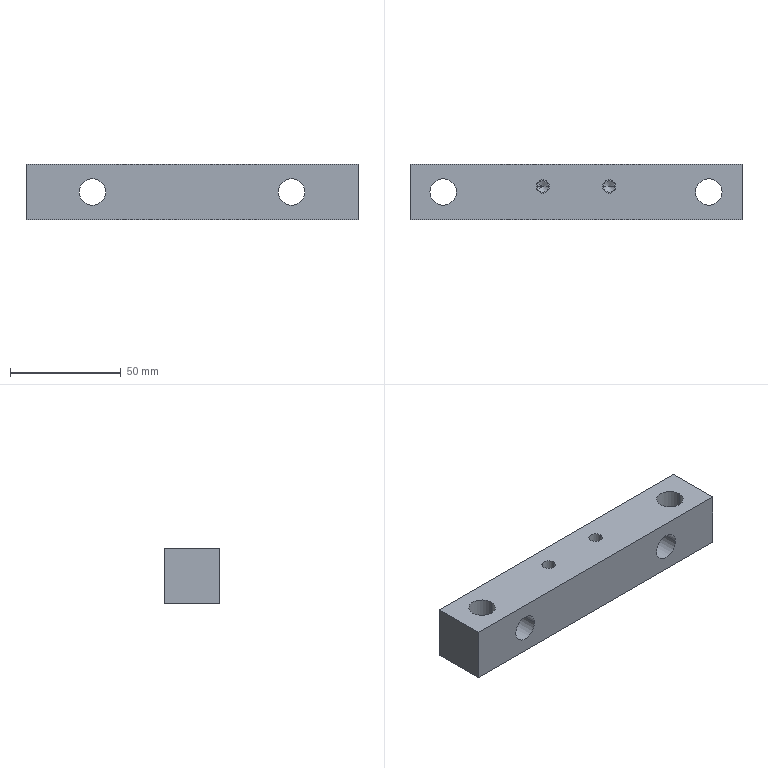Part | STEP file | J013-EBZ05-28-06-Part-1 | 1 solid | 28 faces | box 150 x 25 x 25 mm | volume 81414 mm3 | cylinder 16 | plane 8 | cone 4 | commonest cylinder face diameters 12 x8 5.1 x4 6 x4
STEP:
#1=CARTESIAN_POINT('',(90.,15.,3.468));
#2=VERTEX_POINT('',#1);
#3=CARTESIAN_POINT('',(87.45,15.,5.));
#4=VERTEX_POINT('',#3);
#5=CARTESIAN_POINT('',(87.45,15.,5.));
#6=DIRECTION('',(-0.8572,0.,0.515));
#7=VECTOR('',#6,1000.);
#8=LINE('',#5,#7);
#9=EDGE_CURVE('',#2,#4,#8,.T.);
#10=ORIENTED_EDGE('',*,*,#9,.F.);
#11=CARTESIAN_POINT('',(92.55,15.,5.));
#12=VERTEX_POINT('',#11);
#13=CARTESIAN_POINT('',(92.55,15.,5.));
#14=DIRECTION('',(0.8572,0.,0.515));
#15=VECTOR('',#14,1000.);
#16=LINE('',#13,#15);
#17=EDGE_CURVE('',#2,#12,#16,.T.);
#18=ORIENTED_EDGE('',*,*,#17,.T.);
#19=CARTESIAN_POINT('',(90.,15.,5.));
#20=DIRECTION('',(0.,0.,1.));
#21=DIRECTION('',(-1.,0.,0.));
#22=AXIS2_PLACEMENT_3D('',#19,#20,#21);
#23=CIRCLE('',#22,2.55);
#24=EDGE_CURVE('',#12,#4,#23,.T.);
#25=ORIENTED_EDGE('',*,*,#24,.T.);
#26=EDGE_LOOP('',(#10,#18,#25));
#27=FACE_OUTER_BOUND('',#26,.T.);
#28=CARTESIAN_POINT('',(90.,15.,5.));
#29=DIRECTION('',(0.,0.,1.));
#30=DIRECTION('',(-1.,0.,0.));
#31=AXIS2_PLACEMENT_3D('',#28,#29,#30);
#32=CONICAL_SURFACE('',#31,2.55,1.03);
#33=ADVANCED_FACE('',(#27),#32,.F.);
#34=ORIENTED_EDGE('',*,*,#24,.F.);
#35=CARTESIAN_POINT('',(92.55,15.,13.));
#36=VERTEX_POINT('',#35);
#37=CARTESIAN_POINT('',(92.55,15.,25.));
#38=DIRECTION('',(0.,0.,1.));
#39=VECTOR('',#38,1000.);
#40=LINE('',#37,#39);
#41=EDGE_CURVE('',#12,#36,#40,.T.);
#42=ORIENTED_EDGE('',*,*,#41,.T.);
#43=CARTESIAN_POINT('',(87.45,15.,13.));
#44=VERTEX_POINT('',#43);
#45=CARTESIAN_POINT('',(90.,15.,13.));
#46=DIRECTION('',(0.,0.,1.));
#47=DIRECTION('',(-1.,0.,0.));
#48=AXIS2_PLACEMENT_3D('',#45,#46,#47);
#49=CIRCLE('',#48,2.55);
#50=EDGE_CURVE('',#36,#44,#49,.T.);
#51=ORIENTED_EDGE('',*,*,#50,.T.);
#52=CARTESIAN_POINT('',(87.45,15.,25.));
#53=DIRECTION('',(0.,0.,1.));
#54=VECTOR('',#53,1000.);
#55=LINE('',#52,#54);
#56=EDGE_CURVE('',#4,#44,#55,.T.);
#57=ORIENTED_EDGE('',*,*,#56,.F.);
#58=EDGE_LOOP('',(#34,#42,#51,#57));
#59=FACE_OUTER_BOUND('',#58,.T.);
#60=CARTESIAN_POINT('',(90.,15.,25.));
#61=DIRECTION('',(0.,0.,1.));
#62=DIRECTION('',(-1.,0.,0.));
#63=AXIS2_PLACEMENT_3D('',#60,#61,#62);
#64=CYLINDRICAL_SURFACE('',#63,2.55);
#65=ADVANCED_FACE('',(#59),#64,.F.);
#66=CARTESIAN_POINT('',(93.,15.,13.));
#67=VERTEX_POINT('',#66);
#68=CARTESIAN_POINT('',(87.,15.,13.));
#69=VERTEX_POINT('',#68);
#70=CARTESIAN_POINT('',(90.,15.,13.));
#71=DIRECTION('',(0.,0.,1.));
#72=DIRECTION('',(-1.,0.,0.));
#73=AXIS2_PLACEMENT_3D('',#70,#71,#72);
#74=CIRCLE('',#73,3.);
#75=EDGE_CURVE('',#67,#69,#74,.T.);
#76=ORIENTED_EDGE('',*,*,#75,.F.);
#77=CARTESIAN_POINT('',(93.,15.,25.));
#78=VERTEX_POINT('',#77);
#79=CARTESIAN_POINT('',(93.,15.,25.));
#80=DIRECTION('',(0.,0.,1.));
#81=VECTOR('',#80,1000.);
#82=LINE('',#79,#81);
#83=EDGE_CURVE('',#67,#78,#82,.T.);
#84=ORIENTED_EDGE('',*,*,#83,.T.);
#85=CARTESIAN_POINT('',(87.,15.,25.));
#86=VERTEX_POINT('',#85);
#87=CARTESIAN_POINT('',(90.,15.,25.));
#88=DIRECTION('',(0.,0.,1.));
#89=DIRECTION('',(-1.,0.,0.));
#90=AXIS2_PLACEMENT_3D('',#87,#88,#89);
#91=CIRCLE('',#90,3.);
#92=EDGE_CURVE('',#78,#86,#91,.T.);
#93=ORIENTED_EDGE('',*,*,#92,.T.);
#94=CARTESIAN_POINT('',(87.,15.,25.));
#95=DIRECTION('',(0.,0.,1.));
#96=VECTOR('',#95,1000.);
#97=LINE('',#94,#96);
#98=EDGE_CURVE('',#69,#86,#97,.T.);
#99=ORIENTED_EDGE('',*,*,#98,.F.);
#100=EDGE_LOOP('',(#76,#84,#93,#99));
#101=FACE_OUTER_BOUND('',#100,.T.);
#102=CARTESIAN_POINT('',(90.,15.,25.));
#103=DIRECTION('',(0.,0.,1.));
#104=DIRECTION('',(-1.,0.,0.));
#105=AXIS2_PLACEMENT_3D('',#102,#103,#104);
#106=CYLINDRICAL_SURFACE('',#105,3.);
#107=ADVANCED_FACE('',(#101),#106,.F.);
#108=CARTESIAN_POINT('',(60.,15.,3.468));
#109=VERTEX_POINT('',#108);
#110=CARTESIAN_POINT('',(57.45,15.,5.));
#111=VERTEX_POINT('',#110);
#112=CARTESIAN_POINT('',(57.45,15.,5.));
#113=DIRECTION('',(-0.8572,0.,0.515));
#114=VECTOR('',#113,1000.);
#115=LINE('',#112,#114);
#116=EDGE_CURVE('',#109,#111,#115,.T.);
#117=ORIENTED_EDGE('',*,*,#116,.F.);
#118=CARTESIAN_POINT('',(62.55,15.,5.));
#119=VERTEX_POINT('',#118);
#120=CARTESIAN_POINT('',(62.55,15.,5.));
#121=DIRECTION('',(0.8572,0.,0.515));
#122=VECTOR('',#121,1000.);
#123=LINE('',#120,#122);
#124=EDGE_CURVE('',#109,#119,#123,.T.);
#125=ORIENTED_EDGE('',*,*,#124,.T.);
#126=CARTESIAN_POINT('',(60.,15.,5.));
#127=DIRECTION('',(0.,0.,1.));
#128=DIRECTION('',(-1.,0.,0.));
#129=AXIS2_PLACEMENT_3D('',#126,#127,#128);
#130=CIRCLE('',#129,2.55);
#131=EDGE_CURVE('',#119,#111,#130,.T.);
#132=ORIENTED_EDGE('',*,*,#131,.T.);
#133=EDGE_LOOP('',(#117,#125,#132));
#134=FACE_OUTER_BOUND('',#133,.T.);
#135=CARTESIAN_POINT('',(60.,15.,5.));
#136=DIRECTION('',(0.,0.,1.));
#137=DIRECTION('',(-1.,0.,0.));
#138=AXIS2_PLACEMENT_3D('',#135,#136,#137);
#139=CONICAL_SURFACE('',#138,2.55,1.03);
#140=ADVANCED_FACE('',(#134),#139,.F.);
#141=ORIENTED_EDGE('',*,*,#131,.F.);
#142=CARTESIAN_POINT('',(62.55,15.,13.));
#143=VERTEX_POINT('',#142);
#144=CARTESIAN_POINT('',(62.55,15.,25.));
#145=DIRECTION('',(0.,0.,1.));
#146=VECTOR('',#145,1000.);
#147=LINE('',#144,#146);
#148=EDGE_CURVE('',#119,#143,#147,.T.);
#149=ORIENTED_EDGE('',*,*,#148,.T.);
#150=CARTESIAN_POINT('',(57.45,15.,13.));
#151=VERTEX_POINT('',#150);
#152=CARTESIAN_POINT('',(60.,15.,13.));
#153=DIRECTION('',(0.,0.,1.));
#154=DIRECTION('',(-1.,0.,0.));
#155=AXIS2_PLACEMENT_3D('',#152,#153,#154);
#156=CIRCLE('',#155,2.55);
#157=EDGE_CURVE('',#143,#151,#156,.T.);
#158=ORIENTED_EDGE('',*,*,#157,.T.);
#159=CARTESIAN_POINT('',(57.45,15.,25.));
#160=DIRECTION('',(0.,0.,1.));
#161=VECTOR('',#160,1000.);
#162=LINE('',#159,#161);
#163=EDGE_CURVE('',#111,#151,#162,.T.);
#164=ORIENTED_EDGE('',*,*,#163,.F.);
#165=EDGE_LOOP('',(#141,#149,#158,#164));
#166=FACE_OUTER_BOUND('',#165,.T.);
#167=CARTESIAN_POINT('',(60.,15.,25.));
#168=DIRECTION('',(0.,0.,1.));
#169=DIRECTION('',(-1.,0.,0.));
#170=AXIS2_PLACEMENT_3D('',#167,#168,#169);
#171=CYLINDRICAL_SURFACE('',#170,2.55);
#172=ADVANCED_FACE('',(#166),#171,.F.);
#173=CARTESIAN_POINT('',(63.,15.,13.));
#174=VERTEX_POINT('',#173);
#175=CARTESIAN_POINT('',(57.,15.,13.));
#176=VERTEX_POINT('',#175);
#177=CARTESIAN_POINT('',(60.,15.,13.));
#178=DIRECTION('',(0.,0.,1.));
#179=DIRECTION('',(-1.,0.,0.));
#180=AXIS2_PLACEMENT_3D('',#177,#178,#179);
#181=CIRCLE('',#180,3.);
#182=EDGE_CURVE('',#174,#176,#181,.T.);
#183=ORIENTED_EDGE('',*,*,#182,.F.);
#184=CARTESIAN_POINT('',(63.,15.,25.));
#185=VERTEX_POINT('',#184);
#186=CARTESIAN_POINT('',(63.,15.,25.));
#187=DIRECTION('',(0.,0.,1.));
#188=VECTOR('',#187,1000.);
#189=LINE('',#186,#188);
#190=EDGE_CURVE('',#174,#185,#189,.T.);
#191=ORIENTED_EDGE('',*,*,#190,.T.);
#192=CARTESIAN_POINT('',(57.,15.,25.));
#193=VERTEX_POINT('',#192);
#194=CARTESIAN_POINT('',(60.,15.,25.));
#195=DIRECTION('',(0.,0.,1.));
#196=DIRECTION('',(-1.,0.,0.));
#197=AXIS2_PLACEMENT_3D('',#194,#195,#196);
#198=CIRCLE('',#197,3.);
#199=EDGE_CURVE('',#185,#193,#198,.T.);
#200=ORIENTED_EDGE('',*,*,#199,.T.);
#201=CARTESIAN_POINT('',(57.,15.,25.));
#202=DIRECTION('',(0.,0.,1.));
#203=VECTOR('',#202,1000.);
#204=LINE('',#201,#203);
#205=EDGE_CURVE('',#176,#193,#204,.T.);
#206=ORIENTED_EDGE('',*,*,#205,.F.);
#207=EDGE_LOOP('',(#183,#191,#200,#206));
#208=FACE_OUTER_BOUND('',#207,.T.);
#209=CARTESIAN_POINT('',(60.,15.,25.));
#210=DIRECTION('',(0.,0.,1.));
#211=DIRECTION('',(-1.,0.,0.));
#212=AXIS2_PLACEMENT_3D('',#209,#210,#211);
#213=CYLINDRICAL_SURFACE('',#212,3.);
#214=ADVANCED_FACE('',(#208),#213,.F.);
#215=CARTESIAN_POINT('',(114.,25.,12.5));
#216=VERTEX_POINT('',#215);
#217=CARTESIAN_POINT('',(126.,25.,12.5));
#218=VERTEX_POINT('',#217);
#219=CARTESIAN_POINT('',(120.,25.,12.5));
#220=DIRECTION('',(0.,-1.,0.));
#221=DIRECTION('',(1.,0.,0.));
#222=AXIS2_PLACEMENT_3D('',#219,#220,#221);
#223=CIRCLE('',#222,6.);
#224=EDGE_CURVE('',#216,#218,#223,.T.);
#225=ORIENTED_EDGE('',*,*,#224,.F.);
#226=CARTESIAN_POINT('',(114.,0.,12.5));
#227=VERTEX_POINT('',#226);
#228=CARTESIAN_POINT('',(114.,25.,12.5));
#229=DIRECTION('',(0.,-1.,0.));
#230=VECTOR('',#229,1000.);
#231=LINE('',#228,#230);
#232=EDGE_CURVE('',#216,#227,#231,.T.);
#233=ORIENTED_EDGE('',*,*,#232,.T.);
#234=CARTESIAN_POINT('',(126.,0.,12.5));
#235=VERTEX_POINT('',#234);
#236=CARTESIAN_POINT('',(120.,0.,12.5));
#237=DIRECTION('',(0.,1.,0.));
#238=DIRECTION('',(-1.,0.,0.));
#239=AXIS2_PLACEMENT_3D('',#236,#237,#238);
#240=CIRCLE('',#239,6.);
#241=EDGE_CURVE('',#235,#227,#240,.T.);
#242=ORIENTED_EDGE('',*,*,#241,.F.);
#243=CARTESIAN_POINT('',(126.,25.,12.5));
#244=DIRECTION('',(0.,-1.,0.));
#245=VECTOR('',#244,1000.);
#246=LINE('',#243,#245);
#247=EDGE_CURVE('',#218,#235,#246,.T.);
#248=ORIENTED_EDGE('',*,*,#247,.F.);
#249=EDGE_LOOP('',(#225,#233,#242,#248));
#250=FACE_OUTER_BOUND('',#249,.T.);
#251=CARTESIAN_POINT('',(120.,25.,12.5));
#252=DIRECTION('',(0.,-1.,0.));
#253=DIRECTION('',(1.,0.,0.));
#254=AXIS2_PLACEMENT_3D('',#251,#252,#253);
#255=CYLINDRICAL_SURFACE('',#254,6.);
#256=ADVANCED_FACE('',(#250),#255,.F.);
#257=CARTESIAN_POINT('',(129.,12.5,25.));
#258=VERTEX_POINT('',#257);
#259=CARTESIAN_POINT('',(141.,12.5,25.));
#260=VERTEX_POINT('',#259);
#261=CARTESIAN_POINT('',(135.,12.5,25.));
#262=DIRECTION('',(0.,0.,-1.));
#263=DIRECTION('',(1.,0.,0.));
#264=AXIS2_PLACEMENT_3D('',#261,#262,#263);
#265=CIRCLE('',#264,6.);
#266=EDGE_CURVE('',#258,#260,#265,.T.);
#267=ORIENTED_EDGE('',*,*,#266,.F.);
#268=CARTESIAN_POINT('',(129.,12.5,0.));
#269=VERTEX_POINT('',#268);
#270=CARTESIAN_POINT('',(129.,12.5,25.));
#271=DIRECTION('',(0.,0.,-1.));
#272=VECTOR('',#271,1000.);
#273=LINE('',#270,#272);
#274=EDGE_CURVE('',#258,#269,#273,.T.);
#275=ORIENTED_EDGE('',*,*,#274,.T.);
#276=CARTESIAN_POINT('',(141.,12.5,0.));
#277=VERTEX_POINT('',#276);
#278=CARTESIAN_POINT('',(135.,12.5,0.));
#279=DIRECTION('',(0.,0.,1.));
#280=DIRECTION('',(-1.,0.,0.));
#281=AXIS2_PLACEMENT_3D('',#278,#279,#280);
#282=CIRCLE('',#281,6.);
#283=EDGE_CURVE('',#277,#269,#282,.T.);
#284=ORIENTED_EDGE('',*,*,#283,.F.);
#285=CARTESIAN_POINT('',(141.,12.5,25.));
#286=DIRECTION('',(0.,0.,-1.));
#287=VECTOR('',#286,1000.);
#288=LINE('',#285,#287);
#289=EDGE_CURVE('',#260,#277,#288,.T.);
#290=ORIENTED_EDGE('',*,*,#289,.F.);
#291=EDGE_LOOP('',(#267,#275,#284,#290));
#292=FACE_OUTER_BOUND('',#291,.T.);
#293=CARTESIAN_POINT('',(135.,12.5,25.));
#294=DIRECTION('',(0.,0.,-1.));
#295=DIRECTION('',(1.,0.,0.));
#296=AXIS2_PLACEMENT_3D('',#293,#294,#295);
#297=CYLINDRICAL_SURFACE('',#296,6.);
#298=ADVANCED_FACE('',(#292),#297,.F.);
#299=CARTESIAN_POINT('',(9.,12.5,25.));
#300=VERTEX_POINT('',#299);
#301=CARTESIAN_POINT('',(21.,12.5,25.));
#302=VERTEX_POINT('',#301);
#303=CARTESIAN_POINT('',(15.,12.5,25.));
#304=DIRECTION('',(0.,0.,-1.));
#305=DIRECTION('',(1.,0.,0.));
#306=AXIS2_PLACEMENT_3D('',#303,#304,#305);
#307=CIRCLE('',#306,6.);
#308=EDGE_CURVE('',#300,#302,#307,.T.);
#309=ORIENTED_EDGE('',*,*,#308,.F.);
#310=CARTESIAN_POINT('',(9.,12.5,0.));
#311=VERTEX_POINT('',#310);
#312=CARTESIAN_POINT('',(9.,12.5,25.));
#313=DIRECTION('',(0.,0.,-1.));
#314=VECTOR('',#313,1000.);
#315=LINE('',#312,#314);
#316=EDGE_CURVE('',#300,#311,#315,.T.);
#317=ORIENTED_EDGE('',*,*,#316,.T.);
#318=CARTESIAN_POINT('',(21.,12.5,0.));
#319=VERTEX_POINT('',#318);
#320=CARTESIAN_POINT('',(15.,12.5,0.));
#321=DIRECTION('',(0.,0.,1.));
#322=DIRECTION('',(-1.,0.,0.));
#323=AXIS2_PLACEMENT_3D('',#320,#321,#322);
#324=CIRCLE('',#323,6.);
#325=EDGE_CURVE('',#319,#311,#324,.T.);
#326=ORIENTED_EDGE('',*,*,#325,.F.);
#327=CARTESIAN_POINT('',(21.,12.5,25.));
#328=DIRECTION('',(0.,0.,-1.));
#329=VECTOR('',#328,1000.);
#330=LINE('',#327,#329);
#331=EDGE_CURVE('',#302,#319,#330,.T.);
#332=ORIENTED_EDGE('',*,*,#331,.F.);
#333=EDGE_LOOP('',(#309,#317,#326,#332));
#334=FACE_OUTER_BOUND('',#333,.T.);
#335=CARTESIAN_POINT('',(15.,12.5,25.));
#336=DIRECTION('',(0.,0.,-1.));
#337=DIRECTION('',(1.,0.,0.));
#338=AXIS2_PLACEMENT_3D('',#335,#336,#337);
#339=CYLINDRICAL_SURFACE('',#338,6.);
#340=ADVANCED_FACE('',(#334),#339,.F.);
#341=CARTESIAN_POINT('',(24.,25.,12.5));
#342=VERTEX_POINT('',#341);
#343=CARTESIAN_POINT('',(36.,25.,12.5));
#344=VERTEX_POINT('',#343);
#345=CARTESIAN_POINT('',(30.,25.,12.5));
#346=DIRECTION('',(0.,-1.,0.));
#347=DIRECTION('',(1.,0.,0.));
#348=AXIS2_PLACEMENT_3D('',#345,#346,#347);
#349=CIRCLE('',#348,6.);
#350=EDGE_CURVE('',#342,#344,#349,.T.);
#351=ORIENTED_EDGE('',*,*,#350,.F.);
#352=CARTESIAN_POINT('',(24.,0.,12.5));
#353=VERTEX_POINT('',#352);
#354=CARTESIAN_POINT('',(24.,25.,12.5));
#355=DIRECTION('',(0.,-1.,0.));
#356=VECTOR('',#355,1000.);
#357=LINE('',#354,#356);
#358=EDGE_CURVE('',#342,#353,#357,.T.);
#359=ORIENTED_EDGE('',*,*,#358,.T.);
#360=CARTESIAN_POINT('',(36.,0.,12.5));
#361=VERTEX_POINT('',#360);
#362=CARTESIAN_POINT('',(30.,0.,12.5));
#363=DIRECTION('',(0.,1.,0.));
#364=DIRECTION('',(-1.,0.,0.));
#365=AXIS2_PLACEMENT_3D('',#362,#363,#364);
#366=CIRCLE('',#365,6.);
#367=EDGE_CURVE('',#361,#353,#366,.T.);
#368=ORIENTED_EDGE('',*,*,#367,.F.);
#369=CARTESIAN_POINT('',(36.,25.,12.5));
#370=DIRECTION('',(0.,-1.,0.));
#371=VECTOR('',#370,1000.);
#372=LINE('',#369,#371);
#373=EDGE_CURVE('',#344,#361,#372,.T.);
#374=ORIENTED_EDGE('',*,*,#373,.F.);
#375=EDGE_LOOP('',(#351,#359,#368,#374));
#376=FACE_OUTER_BOUND('',#375,.T.);
#377=CARTESIAN_POINT('',(30.,25.,12.5));
#378=DIRECTION('',(0.,-1.,0.));
#379=DIRECTION('',(1.,0.,0.));
#380=AXIS2_PLACEMENT_3D('',#377,#378,#379);
#381=CYLINDRICAL_SURFACE('',#380,6.);
#382=ADVANCED_FACE('',(#376),#381,.F.);
#383=CARTESIAN_POINT('',(90.,15.,25.));
#384=DIRECTION('',(0.,0.,1.));
#385=DIRECTION('',(-1.,0.,0.));
#386=AXIS2_PLACEMENT_3D('',#383,#384,#385);
#387=CIRCLE('',#386,3.);
#388=EDGE_CURVE('',#86,#78,#387,.T.);
#389=ORIENTED_EDGE('',*,*,#388,.F.);
#390=ORIENTED_EDGE('',*,*,#92,.F.);
#391=EDGE_LOOP('',(#389,#390));
#392=FACE_BOUND('',#391,.T.);
#393=CARTESIAN_POINT('',(60.,15.,25.));
#394=DIRECTION('',(0.,0.,1.));
#395=DIRECTION('',(-1.,0.,0.));
#396=AXIS2_PLACEMENT_3D('',#393,#394,#395);
#397=CIRCLE('',#396,3.);
#398=EDGE_CURVE('',#193,#185,#397,.T.);
#399=ORIENTED_EDGE('',*,*,#398,.F.);
#400=ORIENTED_EDGE('',*,*,#199,.F.);
#401=EDGE_LOOP('',(#399,#400));
#402=FACE_BOUND('',#401,.T.);
#403=CARTESIAN_POINT('',(135.,12.5,25.));
#404=DIRECTION('',(0.,0.,-1.));
#405=DIRECTION('',(1.,0.,0.));
#406=AXIS2_PLACEMENT_3D('',#403,#404,#405);
#407=CIRCLE('',#406,6.);
#408=EDGE_CURVE('',#260,#258,#407,.T.);
#409=ORIENTED_EDGE('',*,*,#408,.T.);
#410=ORIENTED_EDGE('',*,*,#266,.T.);
#411=EDGE_LOOP('',(#409,#410));
#412=FACE_BOUND('',#411,.T.);
#413=CARTESIAN_POINT('',(15.,12.5,25.));
#414=DIRECTION('',(0.,0.,-1.));
#415=DIRECTION('',(1.,0.,0.));
#416=AXIS2_PLACEMENT_3D('',#413,#414,#415);
#417=CIRCLE('',#416,6.);
#418=EDGE_CURVE('',#302,#300,#417,.T.);
#419=ORIENTED_EDGE('',*,*,#418,.T.);
#420=ORIENTED_EDGE('',*,*,#308,.T.);
#421=EDGE_LOOP('',(#419,#420));
#422=FACE_BOUND('',#421,.T.);
#423=CARTESIAN_POINT('',(0.,25.,25.));
#424=VERTEX_POINT('',#423);
#425=CARTESIAN_POINT('',(150.,25.,25.));
#426=VERTEX_POINT('',#425);
#427=CARTESIAN_POINT('',(75.,25.,25.));
#428=DIRECTION('',(1.,0.,0.));
#429=VECTOR('',#428,1000.);
#430=LINE('',#427,#429);
#431=EDGE_CURVE('',#424,#426,#430,.T.);
#432=ORIENTED_EDGE('',*,*,#431,.F.);
#433=CARTESIAN_POINT('',(0.,0.,25.));
#434=VERTEX_POINT('',#433);
#435=CARTESIAN_POINT('',(0.,12.5,25.));
#436=DIRECTION('',(0.,1.,0.));
#437=VECTOR('',#436,1000.);
#438=LINE('',#435,#437);
#439=EDGE_CURVE('',#434,#424,#438,.T.);
#440=ORIENTED_EDGE('',*,*,#439,.F.);
#441=CARTESIAN_POINT('',(150.,0.,25.));
#442=VERTEX_POINT('',#441);
#443=CARTESIAN_POINT('',(75.,0.,25.));
#444=DIRECTION('',(-1.,0.,0.));
#445=VECTOR('',#444,1000.);
#446=LINE('',#443,#445);
#447=EDGE_CURVE('',#442,#434,#446,.T.);
#448=ORIENTED_EDGE('',*,*,#447,.F.);
#449=CARTESIAN_POINT('',(150.,12.5,25.));
#450=DIRECTION('',(0.,-1.,0.));
#451=VECTOR('',#450,1000.);
#452=LINE('',#449,#451);
#453=EDGE_CURVE('',#426,#442,#452,.T.);
#454=ORIENTED_EDGE('',*,*,#453,.F.);
#455=EDGE_LOOP('',(#432,#440,#448,#454));
#456=FACE_OUTER_BOUND('',#455,.T.);
#457=CARTESIAN_POINT('',(75.,12.5,25.));
#458=DIRECTION('',(0.,0.,1.));
#459=DIRECTION('',(-1.,0.,0.));
#460=AXIS2_PLACEMENT_3D('',#457,#458,#459);
#461=PLANE('',#460);
#462=ADVANCED_FACE('',(#392,#402,#412,#422,#456),#461,.T.);
#463=CARTESIAN_POINT('',(120.,25.,12.5));
#464=DIRECTION('',(0.,-1.,0.));
#465=DIRECTION('',(1.,0.,0.));
#466=AXIS2_PLACEMENT_3D('',#463,#464,#465);
#467=CIRCLE('',#466,6.);
#468=EDGE_CURVE('',#218,#216,#467,.T.);
#469=ORIENTED_EDGE('',*,*,#468,.T.);
#470=ORIENTED_EDGE('',*,*,#224,.T.);
#471=EDGE_LOOP('',(#469,#470));
#472=FACE_BOUND('',#471,.T.);
#473=CARTESIAN_POINT('',(30.,25.,12.5));
#474=DIRECTION('',(0.,-1.,0.));
#475=DIRECTION('',(1.,0.,0.));
#476=AXIS2_PLACEMENT_3D('',#473,#474,#475);
#477=CIRCLE('',#476,6.);
#478=EDGE_CURVE('',#344,#342,#477,.T.);
#479=ORIENTED_EDGE('',*,*,#478,.T.);
#480=ORIENTED_EDGE('',*,*,#350,.T.);
#481=EDGE_LOOP('',(#479,#480));
#482=FACE_BOUND('',#481,.T.);
#483=CARTESIAN_POINT('',(0.,25.,0.));
#484=VERTEX_POINT('',#483);
#485=CARTESIAN_POINT('',(0.,25.,0.));
#486=DIRECTION('',(0.,0.,1.));
#487=VECTOR('',#486,1000.);
#488=LINE('',#485,#487);
#489=EDGE_CURVE('',#484,#424,#488,.T.);
#490=ORIENTED_EDGE('',*,*,#489,.T.);
#491=ORIENTED_EDGE('',*,*,#431,.T.);
#492=CARTESIAN_POINT('',(150.,25.,0.));
#493=VERTEX_POINT('',#492);
#494=CARTESIAN_POINT('',(150.,25.,0.));
#495=DIRECTION('',(0.,0.,1.));
#496=VECTOR('',#495,1000.);
#497=LINE('',#494,#496);
#498=EDGE_CURVE('',#493,#426,#497,.T.);
#499=ORIENTED_EDGE('',*,*,#498,.F.);
#500=CARTESIAN_POINT('',(75.,25.,0.));
#501=DIRECTION('',(-1.,0.,0.));
#502=VECTOR('',#501,1000.);
#503=LINE('',#500,#502);
#504=EDGE_CURVE('',#493,#484,#503,.T.);
#505=ORIENTED_EDGE('',*,*,#504,.T.);
#506=EDGE_LOOP('',(#490,#491,#499,#505));
#507=FACE_OUTER_BOUND('',#506,.T.);
#508=CARTESIAN_POINT('',(75.,25.,0.));
#509=DIRECTION('',(0.,1.,0.));
#510=DIRECTION('',(0.,0.,-1.));
#511=AXIS2_PLACEMENT_3D('',#508,#509,#510);
#512=PLANE('',#511);
#513=ADVANCED_FACE('',(#472,#482,#507),#512,.T.);
#514=ORIENTED_EDGE('',*,*,#498,.T.);
#515=ORIENTED_EDGE('',*,*,#453,.T.);
#516=CARTESIAN_POINT('',(150.,0.,0.));
#517=VERTEX_POINT('',#516);
#518=CARTESIAN_POINT('',(150.,0.,0.));
#519=DIRECTION('',(0.,0.,1.));
#520=VECTOR('',#519,1000.);
#521=LINE('',#518,#520);
#522=EDGE_CURVE('',#517,#442,#521,.T.);
#523=ORIENTED_EDGE('',*,*,#522,.F.);
#524=CARTESIAN_POINT('',(150.,12.5,0.));
#525=DIRECTION('',(0.,1.,0.));
#526=VECTOR('',#525,1000.);
#527=LINE('',#524,#526);
#528=EDGE_CURVE('',#517,#493,#527,.T.);
#529=ORIENTED_EDGE('',*,*,#528,.T.);
#530=EDGE_LOOP('',(#514,#515,#523,#529));
#531=FACE_OUTER_BOUND('',#530,.T.);
#532=CARTESIAN_POINT('',(150.,12.5,0.));
#533=DIRECTION('',(1.,0.,0.));
#534=DIRECTION('',(0.,0.,1.));
#535=AXIS2_PLACEMENT_3D('',#532,#533,#534);
#536=PLANE('',#535);
#537=ADVANCED_FACE('',(#531),#536,.T.);
#538=ORIENTED_EDGE('',*,*,#241,.T.);
#539=CARTESIAN_POINT('',(120.,0.,12.5));
#540=DIRECTION('',(0.,1.,0.));
#541=DIRECTION('',(-1.,0.,0.));
#542=AXIS2_PLACEMENT_3D('',#539,#540,#541);
#543=CIRCLE('',#542,6.);
#544=EDGE_CURVE('',#227,#235,#543,.T.);
#545=ORIENTED_EDGE('',*,*,#544,.T.);
#546=EDGE_LOOP('',(#538,#545));
#547=FACE_BOUND('',#546,.T.);
#548=ORIENTED_EDGE('',*,*,#367,.T.);
#549=CARTESIAN_POINT('',(30.,0.,12.5));
#550=DIRECTION('',(0.,1.,0.));
#551=DIRECTION('',(-1.,0.,0.));
#552=AXIS2_PLACEMENT_3D('',#549,#550,#551);
#553=CIRCLE('',#552,6.);
#554=EDGE_CURVE('',#353,#361,#553,.T.);
#555=ORIENTED_EDGE('',*,*,#554,.T.);
#556=EDGE_LOOP('',(#548,#555));
#557=FACE_BOUND('',#556,.T.);
#558=ORIENTED_EDGE('',*,*,#522,.T.);
#559=ORIENTED_EDGE('',*,*,#447,.T.);
#560=CARTESIAN_POINT('',(0.,0.,0.));
#561=VERTEX_POINT('',#560);
#562=CARTESIAN_POINT('',(0.,0.,0.));
#563=DIRECTION('',(0.,0.,1.));
#564=VECTOR('',#563,1000.);
#565=LINE('',#562,#564);
#566=EDGE_CURVE('',#561,#434,#565,.T.);
#567=ORIENTED_EDGE('',*,*,#566,.F.);
#568=CARTESIAN_POINT('',(75.,0.,0.));
#569=DIRECTION('',(1.,0.,0.));
#570=VECTOR('',#569,1000.);
#571=LINE('',#568,#570);
#572=EDGE_CURVE('',#561,#517,#571,.T.);
#573=ORIENTED_EDGE('',*,*,#572,.T.);
#574=EDGE_LOOP('',(#558,#559,#567,#573));
#575=FACE_OUTER_BOUND('',#574,.T.);
#576=CARTESIAN_POINT('',(75.,0.,0.));
#577=DIRECTION('',(0.,-1.,0.));
#578=DIRECTION('',(0.,0.,1.));
#579=AXIS2_PLACEMENT_3D('',#576,#577,#578);
#580=PLANE('',#579);
#581=ADVANCED_FACE('',(#547,#557,#575),#580,.T.);
#582=ORIENTED_EDGE('',*,*,#283,.T.);
#583=CARTESIAN_POINT('',(135.,12.5,0.));
#584=DIRECTION('',(0.,0.,1.));
#585=DIRECTION('',(-1.,0.,0.));
#586=AXIS2_PLACEMENT_3D('',#583,#584,#585);
#587=CIRCLE('',#586,6.);
#588=EDGE_CURVE('',#269,#277,#587,.T.);
#589=ORIENTED_EDGE('',*,*,#588,.T.);
#590=EDGE_LOOP('',(#582,#589));
#591=FACE_BOUND('',#590,.T.);
#592=ORIENTED_EDGE('',*,*,#325,.T.);
#593=CARTESIAN_POINT('',(15.,12.5,0.));
#594=DIRECTION('',(0.,0.,1.));
#595=DIRECTION('',(-1.,0.,0.));
#596=AXIS2_PLACEMENT_3D('',#593,#594,#595);
#597=CIRCLE('',#596,6.);
#598=EDGE_CURVE('',#311,#319,#597,.T.);
#599=ORIENTED_EDGE('',*,*,#598,.T.);
#600=EDGE_LOOP('',(#592,#599));
#601=FACE_BOUND('',#600,.T.);
#602=CARTESIAN_POINT('',(0.,12.5,0.));
#603=DIRECTION('',(0.,-1.,0.));
#604=VECTOR('',#603,1000.);
#605=LINE('',#602,#604);
#606=EDGE_CURVE('',#484,#561,#605,.T.);
#607=ORIENTED_EDGE('',*,*,#606,.F.);
#608=ORIENTED_EDGE('',*,*,#504,.F.);
#609=ORIENTED_EDGE('',*,*,#528,.F.);
#610=ORIENTED_EDGE('',*,*,#572,.F.);
#611=EDGE_LOOP('',(#607,#608,#609,#610));
#612=FACE_OUTER_BOUND('',#611,.T.);
#613=CARTESIAN_POINT('',(75.,12.5,0.));
#614=DIRECTION('',(0.,0.,-1.));
#615=DIRECTION('',(1.,0.,0.));
#616=AXIS2_PLACEMENT_3D('',#613,#614,#615);
#617=PLANE('',#616);
#618=ADVANCED_FACE('',(#591,#601,#612),#617,.T.);
#619=ORIENTED_EDGE('',*,*,#606,.T.);
#620=ORIENTED_EDGE('',*,*,#566,.T.);
#621=ORIENTED_EDGE('',*,*,#439,.T.);
#622=ORIENTED_EDGE('',*,*,#489,.F.);
#623=EDGE_LOOP('',(#619,#620,#621,#622));
#624=FACE_OUTER_BOUND('',#623,.T.);
#625=CARTESIAN_POINT('',(0.,12.5,0.));
#626=DIRECTION('',(-1.,0.,0.));
#627=DIRECTION('',(0.,0.,-1.));
#628=AXIS2_PLACEMENT_3D('',#625,#626,#627);
#629=PLANE('',#628);
#630=ADVANCED_FACE('',(#624),#629,.T.);
#631=ORIENTED_EDGE('',*,*,#358,.F.);
#632=ORIENTED_EDGE('',*,*,#478,.F.);
#633=ORIENTED_EDGE('',*,*,#373,.T.);
#634=ORIENTED_EDGE('',*,*,#554,.F.);
#635=EDGE_LOOP('',(#631,#632,#633,#634));
#636=FACE_OUTER_BOUND('',#635,.T.);
#637=CARTESIAN_POINT('',(30.,25.,12.5));
#638=DIRECTION('',(0.,-1.,0.));
#639=DIRECTION('',(1.,0.,0.));
#640=AXIS2_PLACEMENT_3D('',#637,#638,#639);
#641=CYLINDRICAL_SURFACE('',#640,6.);
#642=ADVANCED_FACE('',(#636),#641,.F.);
#643=ORIENTED_EDGE('',*,*,#316,.F.);
#644=ORIENTED_EDGE('',*,*,#418,.F.);
#645=ORIENTED_EDGE('',*,*,#331,.T.);
#646=ORIENTED_EDGE('',*,*,#598,.F.);
#647=EDGE_LOOP('',(#643,#644,#645,#646));
#648=FACE_OUTER_BOUND('',#647,.T.);
#649=CARTESIAN_POINT('',(15.,12.5,25.));
#650=DIRECTION('',(0.,0.,-1.));
#651=DIRECTION('',(1.,0.,0.));
#652=AXIS2_PLACEMENT_3D('',#649,#650,#651);
#653=CYLINDRICAL_SURFACE('',#652,6.);
#654=ADVANCED_FACE('',(#648),#653,.F.);
#655=ORIENTED_EDGE('',*,*,#274,.F.);
#656=ORIENTED_EDGE('',*,*,#408,.F.);
#657=ORIENTED_EDGE('',*,*,#289,.T.);
#658=ORIENTED_EDGE('',*,*,#588,.F.);
#659=EDGE_LOOP('',(#655,#656,#657,#658));
#660=FACE_OUTER_BOUND('',#659,.T.);
#661=CARTESIAN_POINT('',(135.,12.5,25.));
#662=DIRECTION('',(0.,0.,-1.));
#663=DIRECTION('',(1.,0.,0.));
#664=AXIS2_PLACEMENT_3D('',#661,#662,#663);
#665=CYLINDRICAL_SURFACE('',#664,6.);
#666=ADVANCED_FACE('',(#660),#665,.F.);
#667=ORIENTED_EDGE('',*,*,#232,.F.);
#668=ORIENTED_EDGE('',*,*,#468,.F.);
#669=ORIENTED_EDGE('',*,*,#247,.T.);
#670=ORIENTED_EDGE('',*,*,#544,.F.);
#671=EDGE_LOOP('',(#667,#668,#669,#670));
#672=FACE_OUTER_BOUND('',#671,.T.);
#673=CARTESIAN_POINT('',(120.,25.,12.5));
#674=DIRECTION('',(0.,-1.,0.));
#675=DIRECTION('',(1.,0.,0.));
#676=AXIS2_PLACEMENT_3D('',#673,#674,#675);
#677=CYLINDRICAL_SURFACE('',#676,6.);
#678=ADVANCED_FACE('',(#672),#677,.F.);
#679=ORIENTED_EDGE('',*,*,#190,.F.);
#680=CARTESIAN_POINT('',(60.,15.,13.));
#681=DIRECTION('',(0.,0.,1.));
#682=DIRECTION('',(-1.,0.,0.));
#683=AXIS2_PLACEMENT_3D('',#680,#681,#682);
#684=CIRCLE('',#683,3.);
#685=EDGE_CURVE('',#176,#174,#684,.T.);
#686=ORIENTED_EDGE('',*,*,#685,.F.);
#687=ORIENTED_EDGE('',*,*,#205,.T.);
#688=ORIENTED_EDGE('',*,*,#398,.T.);
#689=EDGE_LOOP('',(#679,#686,#687,#688));
#690=FACE_OUTER_BOUND('',#689,.T.);
#691=CARTESIAN_POINT('',(60.,15.,25.));
#692=DIRECTION('',(0.,0.,1.));
#693=DIRECTION('',(-1.,0.,0.));
#694=AXIS2_PLACEMENT_3D('',#691,#692,#693);
#695=CYLINDRICAL_SURFACE('',#694,3.);
#696=ADVANCED_FACE('',(#690),#695,.F.);
#697=CARTESIAN_POINT('',(60.,15.,13.));
#698=DIRECTION('',(0.,0.,1.));
#699=DIRECTION('',(-1.,0.,0.));
#700=AXIS2_PLACEMENT_3D('',#697,#698,#699);
#701=CIRCLE('',#700,2.55);
#702=EDGE_CURVE('',#151,#143,#701,.T.);
#703=ORIENTED_EDGE('',*,*,#702,.F.);
#704=ORIENTED_EDGE('',*,*,#157,.F.);
#705=EDGE_LOOP('',(#703,#704));
#706=FACE_BOUND('',#705,.T.);
#707=ORIENTED_EDGE('',*,*,#685,.T.);
#708=ORIENTED_EDGE('',*,*,#182,.T.);
#709=EDGE_LOOP('',(#707,#708));
#710=FACE_OUTER_BOUND('',#709,.T.);
#711=CARTESIAN_POINT('',(63.,15.,13.));
#712=DIRECTION('',(0.,0.,-1.));
#713=DIRECTION('',(1.,0.,0.));
#714=AXIS2_PLACEMENT_3D('',#711,#712,#713);
#715=PLANE('',#714);
#716=ADVANCED_FACE('',(#706,#710),#715,.F.);
#717=ORIENTED_EDGE('',*,*,#148,.F.);
#718=CARTESIAN_POINT('',(60.,15.,5.));
#719=DIRECTION('',(0.,0.,1.));
#720=DIRECTION('',(-1.,0.,0.));
#721=AXIS2_PLACEMENT_3D('',#718,#719,#720);
#722=CIRCLE('',#721,2.55);
#723=EDGE_CURVE('',#111,#119,#722,.T.);
#724=ORIENTED_EDGE('',*,*,#723,.F.);
#725=ORIENTED_EDGE('',*,*,#163,.T.);
#726=ORIENTED_EDGE('',*,*,#702,.T.);
#727=EDGE_LOOP('',(#717,#724,#725,#726));
#728=FACE_OUTER_BOUND('',#727,.T.);
#729=CARTESIAN_POINT('',(60.,15.,25.));
#730=DIRECTION('',(0.,0.,1.));
#731=DIRECTION('',(-1.,0.,0.));
#732=AXIS2_PLACEMENT_3D('',#729,#730,#731);
#733=CYLINDRICAL_SURFACE('',#732,2.55);
#734=ADVANCED_FACE('',(#728),#733,.F.);
#735=ORIENTED_EDGE('',*,*,#124,.F.);
#736=ORIENTED_EDGE('',*,*,#116,.T.);
#737=ORIENTED_EDGE('',*,*,#723,.T.);
#738=EDGE_LOOP('',(#735,#736,#737));
#739=FACE_OUTER_BOUND('',#738,.T.);
#740=CARTESIAN_POINT('',(60.,15.,5.));
#741=DIRECTION('',(0.,0.,1.));
#742=DIRECTION('',(-1.,0.,0.));
#743=AXIS2_PLACEMENT_3D('',#740,#741,#742);
#744=CONICAL_SURFACE('',#743,2.55,1.03);
#745=ADVANCED_FACE('',(#739),#744,.F.);
#746=ORIENTED_EDGE('',*,*,#83,.F.);
#747=CARTESIAN_POINT('',(90.,15.,13.));
#748=DIRECTION('',(0.,0.,1.));
#749=DIRECTION('',(-1.,0.,0.));
#750=AXIS2_PLACEMENT_3D('',#747,#748,#749);
#751=CIRCLE('',#750,3.);
#752=EDGE_CURVE('',#69,#67,#751,.T.);
#753=ORIENTED_EDGE('',*,*,#752,.F.);
#754=ORIENTED_EDGE('',*,*,#98,.T.);
#755=ORIENTED_EDGE('',*,*,#388,.T.);
#756=EDGE_LOOP('',(#746,#753,#754,#755));
#757=FACE_OUTER_BOUND('',#756,.T.);
#758=CARTESIAN_POINT('',(90.,15.,25.));
#759=DIRECTION('',(0.,0.,1.));
#760=DIRECTION('',(-1.,0.,0.));
#761=AXIS2_PLACEMENT_3D('',#758,#759,#760);
#762=CYLINDRICAL_SURFACE('',#761,3.);
#763=ADVANCED_FACE('',(#757),#762,.F.);
#764=CARTESIAN_POINT('',(90.,15.,13.));
#765=DIRECTION('',(0.,0.,1.));
#766=DIRECTION('',(-1.,0.,0.));
#767=AXIS2_PLACEMENT_3D('',#764,#765,#766);
#768=CIRCLE('',#767,2.55);
#769=EDGE_CURVE('',#44,#36,#768,.T.);
#770=ORIENTED_EDGE('',*,*,#769,.F.);
#771=ORIENTED_EDGE('',*,*,#50,.F.);
#772=EDGE_LOOP('',(#770,#771));
#773=FACE_BOUND('',#772,.T.);
#774=ORIENTED_EDGE('',*,*,#752,.T.);
#775=ORIENTED_EDGE('',*,*,#75,.T.);
#776=EDGE_LOOP('',(#774,#775));
#777=FACE_OUTER_BOUND('',#776,.T.);
#778=CARTESIAN_POINT('',(93.,15.,13.));
#779=DIRECTION('',(0.,0.,-1.));
#780=DIRECTION('',(1.,0.,0.));
#781=AXIS2_PLACEMENT_3D('',#778,#779,#780);
#782=PLANE('',#781);
#783=ADVANCED_FACE('',(#773,#777),#782,.F.);
#784=ORIENTED_EDGE('',*,*,#41,.F.);
#785=CARTESIAN_POINT('',(90.,15.,5.));
#786=DIRECTION('',(0.,0.,1.));
#787=DIRECTION('',(-1.,0.,0.));
#788=AXIS2_PLACEMENT_3D('',#785,#786,#787);
#789=CIRCLE('',#788,2.55);
#790=EDGE_CURVE('',#4,#12,#789,.T.);
#791=ORIENTED_EDGE('',*,*,#790,.F.);
#792=ORIENTED_EDGE('',*,*,#56,.T.);
#793=ORIENTED_EDGE('',*,*,#769,.T.);
#794=EDGE_LOOP('',(#784,#791,#792,#793));
#795=FACE_OUTER_BOUND('',#794,.T.);
#796=CARTESIAN_POINT('',(90.,15.,25.));
#797=DIRECTION('',(0.,0.,1.));
#798=DIRECTION('',(-1.,0.,0.));
#799=AXIS2_PLACEMENT_3D('',#796,#797,#798);
#800=CYLINDRICAL_SURFACE('',#799,2.55);
#801=ADVANCED_FACE('',(#795),#800,.F.);
#802=ORIENTED_EDGE('',*,*,#17,.F.);
#803=ORIENTED_EDGE('',*,*,#9,.T.);
#804=ORIENTED_EDGE('',*,*,#790,.T.);
#805=EDGE_LOOP('',(#802,#803,#804));
#806=FACE_OUTER_BOUND('',#805,.T.);
#807=CARTESIAN_POINT('',(90.,15.,5.));
#808=DIRECTION('',(0.,0.,1.));
#809=DIRECTION('',(-1.,0.,0.));
#810=AXIS2_PLACEMENT_3D('',#807,#808,#809);
#811=CONICAL_SURFACE('',#810,2.55,1.03);
#812=ADVANCED_FACE('',(#806),#811,.F.);
#813=CLOSED_SHELL('',(#33,#65,#107,#140,#172,#214,#256,#298,#340,#382,#462,#513,#537,#581,#618,#630,#642,#654,#666,#678,#696,#716,#734,#745,#763,#783,#801,#812));
#814=MANIFOLD_SOLID_BREP('',#813);
#815=CARTESIAN_POINT('',(0.,0.,0.));
#816=DIRECTION('',(0.,0.,1.));
#817=DIRECTION('',(1.,0.,0.));
#818=AXIS2_PLACEMENT_3D('',#815,#816,#817);
#819=(LENGTH_UNIT()NAMED_UNIT(*)SI_UNIT(.MILLI.,.METRE.));
#820=UNCERTAINTY_MEASURE_WITH_UNIT(LENGTH_MEASURE(0.00001),#819,'','');
#821=(NAMED_UNIT(*)PLANE_ANGLE_UNIT()SI_UNIT($,.RADIAN.));
#822=(NAMED_UNIT(*)SI_UNIT($,.STERADIAN.)SOLID_ANGLE_UNIT());
#823=(GEOMETRIC_REPRESENTATION_CONTEXT(3)GLOBAL_UNCERTAINTY_ASSIGNED_CONTEXT((#820))GLOBAL_UNIT_ASSIGNED_CONTEXT((#819,#821,#822))REPRESENTATION_CONTEXT('',''));
#824=ADVANCED_BREP_SHAPE_REPRESENTATION('',(#814,#818),#823);